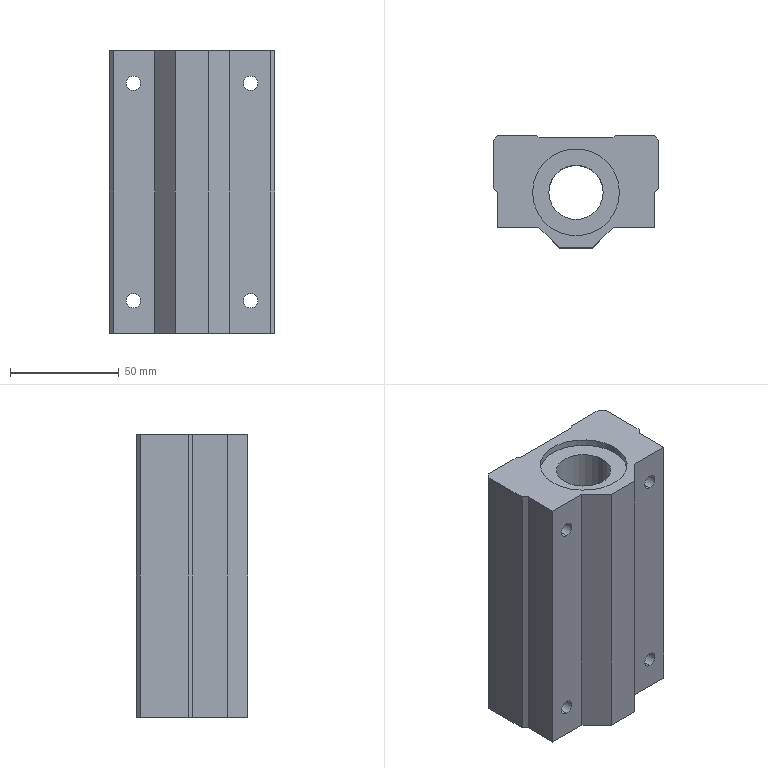Part | SolidWorks | features BaseBody 1 | 1 solid | 44 faces | box 76 x 51.5 x 130 mm | volume 357296 mm3 | plane 22 | cylinder 14 | cone 8 | commonest cylinder face diameters 6.647 x8 40 x4 25 x2
STEP:
#1=CARTESIAN_POINT('',(-12.5,0.,-127.));
#2=VERTEX_POINT('',#1);
#3=CARTESIAN_POINT('',(12.5,0.,-127.));
#4=VERTEX_POINT('',#3);
#5=CARTESIAN_POINT('',(0.,0.,-127.));
#6=DIRECTION('',(0.,0.,1.));
#7=DIRECTION('',(1.,0.,0.));
#8=AXIS2_PLACEMENT_3D('',#5,#6,#7);
#9=CIRCLE('',#8,12.5);
#10=EDGE_CURVE('',#2,#4,#9,.T.);
#11=ORIENTED_EDGE('',*,*,#10,.F.);
#12=CARTESIAN_POINT('',(-12.5,0.,-3.));
#13=VERTEX_POINT('',#12);
#14=CARTESIAN_POINT('',(-12.5,0.,-130.));
#15=DIRECTION('',(0.,0.,1.));
#16=VECTOR('',#15,1000.);
#17=LINE('',#14,#16);
#18=EDGE_CURVE('',#2,#13,#17,.T.);
#19=ORIENTED_EDGE('',*,*,#18,.T.);
#20=CARTESIAN_POINT('',(12.5,0.,-3.));
#21=VERTEX_POINT('',#20);
#22=CARTESIAN_POINT('',(0.,0.,-3.));
#23=DIRECTION('',(0.,0.,-1.));
#24=DIRECTION('',(1.,0.,0.));
#25=AXIS2_PLACEMENT_3D('',#22,#23,#24);
#26=CIRCLE('',#25,12.5);
#27=EDGE_CURVE('',#21,#13,#26,.T.);
#28=ORIENTED_EDGE('',*,*,#27,.F.);
#29=CARTESIAN_POINT('',(12.5,0.,-130.));
#30=DIRECTION('',(0.,0.,1.));
#31=VECTOR('',#30,1000.);
#32=LINE('',#29,#31);
#33=EDGE_CURVE('',#4,#21,#32,.T.);
#34=ORIENTED_EDGE('',*,*,#33,.F.);
#35=EDGE_LOOP('',(#11,#19,#28,#34));
#36=FACE_OUTER_BOUND('',#35,.T.);
#37=CARTESIAN_POINT('',(0.,0.,-130.));
#38=DIRECTION('',(0.,0.,1.));
#39=DIRECTION('',(1.,0.,0.));
#40=AXIS2_PLACEMENT_3D('',#37,#38,#39);
#41=CYLINDRICAL_SURFACE('',#40,12.5);
#42=ADVANCED_FACE('',(#36),#41,.F.);
#43=CARTESIAN_POINT('',(-20.,0.,-3.));
#44=VERTEX_POINT('',#43);
#45=CARTESIAN_POINT('',(20.,0.,-3.));
#46=VERTEX_POINT('',#45);
#47=CARTESIAN_POINT('',(0.,0.,-3.));
#48=DIRECTION('',(0.,0.,1.));
#49=DIRECTION('',(1.,0.,0.));
#50=AXIS2_PLACEMENT_3D('',#47,#48,#49);
#51=CIRCLE('',#50,20.);
#52=EDGE_CURVE('',#44,#46,#51,.T.);
#53=ORIENTED_EDGE('',*,*,#52,.F.);
#54=CARTESIAN_POINT('',(-20.,0.,0.));
#55=VERTEX_POINT('',#54);
#56=CARTESIAN_POINT('',(-20.,0.,-130.));
#57=DIRECTION('',(0.,0.,1.));
#58=VECTOR('',#57,1000.);
#59=LINE('',#56,#58);
#60=EDGE_CURVE('',#44,#55,#59,.T.);
#61=ORIENTED_EDGE('',*,*,#60,.T.);
#62=CARTESIAN_POINT('',(20.,0.,0.));
#63=VERTEX_POINT('',#62);
#64=CARTESIAN_POINT('',(0.,0.,0.));
#65=DIRECTION('',(0.,0.,-1.));
#66=DIRECTION('',(1.,0.,0.));
#67=AXIS2_PLACEMENT_3D('',#64,#65,#66);
#68=CIRCLE('',#67,20.);
#69=EDGE_CURVE('',#63,#55,#68,.T.);
#70=ORIENTED_EDGE('',*,*,#69,.F.);
#71=CARTESIAN_POINT('',(20.,0.,-130.));
#72=DIRECTION('',(0.,0.,1.));
#73=VECTOR('',#72,1000.);
#74=LINE('',#71,#73);
#75=EDGE_CURVE('',#46,#63,#74,.T.);
#76=ORIENTED_EDGE('',*,*,#75,.F.);
#77=EDGE_LOOP('',(#53,#61,#70,#76));
#78=FACE_OUTER_BOUND('',#77,.T.);
#79=CARTESIAN_POINT('',(0.,0.,-130.));
#80=DIRECTION('',(0.,0.,1.));
#81=DIRECTION('',(1.,0.,0.));
#82=AXIS2_PLACEMENT_3D('',#79,#80,#81);
#83=CYLINDRICAL_SURFACE('',#82,20.);
#84=ADVANCED_FACE('',(#78),#83,.F.);
#85=CARTESIAN_POINT('',(-20.,0.,-130.));
#86=VERTEX_POINT('',#85);
#87=CARTESIAN_POINT('',(20.,0.,-130.));
#88=VERTEX_POINT('',#87);
#89=CARTESIAN_POINT('',(0.,0.,-130.));
#90=DIRECTION('',(0.,0.,1.));
#91=DIRECTION('',(1.,0.,0.));
#92=AXIS2_PLACEMENT_3D('',#89,#90,#91);
#93=CIRCLE('',#92,20.);
#94=EDGE_CURVE('',#86,#88,#93,.T.);
#95=ORIENTED_EDGE('',*,*,#94,.F.);
#96=CARTESIAN_POINT('',(-20.,0.,-127.));
#97=VERTEX_POINT('',#96);
#98=CARTESIAN_POINT('',(-20.,0.,-130.));
#99=DIRECTION('',(0.,0.,1.));
#100=VECTOR('',#99,1000.);
#101=LINE('',#98,#100);
#102=EDGE_CURVE('',#86,#97,#101,.T.);
#103=ORIENTED_EDGE('',*,*,#102,.T.);
#104=CARTESIAN_POINT('',(20.,0.,-127.));
#105=VERTEX_POINT('',#104);
#106=CARTESIAN_POINT('',(0.,0.,-127.));
#107=DIRECTION('',(0.,0.,-1.));
#108=DIRECTION('',(1.,0.,0.));
#109=AXIS2_PLACEMENT_3D('',#106,#107,#108);
#110=CIRCLE('',#109,20.);
#111=EDGE_CURVE('',#105,#97,#110,.T.);
#112=ORIENTED_EDGE('',*,*,#111,.F.);
#113=CARTESIAN_POINT('',(20.,0.,-130.));
#114=DIRECTION('',(0.,0.,1.));
#115=VECTOR('',#114,1000.);
#116=LINE('',#113,#115);
#117=EDGE_CURVE('',#88,#105,#116,.T.);
#118=ORIENTED_EDGE('',*,*,#117,.F.);
#119=EDGE_LOOP('',(#95,#103,#112,#118));
#120=FACE_OUTER_BOUND('',#119,.T.);
#121=CARTESIAN_POINT('',(0.,0.,-130.));
#122=DIRECTION('',(0.,0.,1.));
#123=DIRECTION('',(1.,0.,0.));
#124=AXIS2_PLACEMENT_3D('',#121,#122,#123);
#125=CYLINDRICAL_SURFACE('',#124,20.);
#126=ADVANCED_FACE('',(#120),#125,.F.);
#127=CARTESIAN_POINT('',(-27.,25.323,-118.323));
#128=VERTEX_POINT('',#127);
#129=CARTESIAN_POINT('',(-27.,25.323,-111.677));
#130=VERTEX_POINT('',#129);
#131=CARTESIAN_POINT('',(-27.,25.323,-115.));
#132=DIRECTION('',(0.,1.,0.));
#133=DIRECTION('',(0.,0.,1.));
#134=AXIS2_PLACEMENT_3D('',#131,#132,#133);
#135=CIRCLE('',#134,3.323);
#136=EDGE_CURVE('',#128,#130,#135,.T.);
#137=ORIENTED_EDGE('',*,*,#136,.F.);
#138=CARTESIAN_POINT('',(-27.,26.,-119.));
#139=VERTEX_POINT('',#138);
#140=CARTESIAN_POINT('',(-27.,26.,-119.));
#141=DIRECTION('',(0.,0.7071,-0.7071));
#142=VECTOR('',#141,1000.);
#143=LINE('',#140,#142);
#144=EDGE_CURVE('',#128,#139,#143,.T.);
#145=ORIENTED_EDGE('',*,*,#144,.T.);
#146=CARTESIAN_POINT('',(-27.,26.,-111.));
#147=VERTEX_POINT('',#146);
#148=CARTESIAN_POINT('',(-27.,26.,-115.));
#149=DIRECTION('',(0.,-1.,0.));
#150=DIRECTION('',(0.,0.,1.));
#151=AXIS2_PLACEMENT_3D('',#148,#149,#150);
#152=CIRCLE('',#151,4.);
#153=EDGE_CURVE('',#147,#139,#152,.T.);
#154=ORIENTED_EDGE('',*,*,#153,.F.);
#155=CARTESIAN_POINT('',(-27.,26.,-111.));
#156=DIRECTION('',(0.,0.7071,0.7071));
#157=VECTOR('',#156,1000.);
#158=LINE('',#155,#157);
#159=EDGE_CURVE('',#130,#147,#158,.T.);
#160=ORIENTED_EDGE('',*,*,#159,.F.);
#161=EDGE_LOOP('',(#137,#145,#154,#160));
#162=FACE_OUTER_BOUND('',#161,.T.);
#163=CARTESIAN_POINT('',(-27.,26.,-115.));
#164=DIRECTION('',(0.,1.,0.));
#165=DIRECTION('',(0.,0.,1.));
#166=AXIS2_PLACEMENT_3D('',#163,#164,#165);
#167=CONICAL_SURFACE('',#166,4.,0.7854);
#168=ADVANCED_FACE('',(#162),#167,.F.);
#169=CARTESIAN_POINT('',(-27.,25.324,-18.324));
#170=VERTEX_POINT('',#169);
#171=CARTESIAN_POINT('',(-27.,25.324,-11.676));
#172=VERTEX_POINT('',#171);
#173=CARTESIAN_POINT('',(-27.,25.324,-15.));
#174=DIRECTION('',(0.,1.,0.));
#175=DIRECTION('',(0.,0.,1.));
#176=AXIS2_PLACEMENT_3D('',#173,#174,#175);
#177=CIRCLE('',#176,3.324);
#178=EDGE_CURVE('',#170,#172,#177,.T.);
#179=ORIENTED_EDGE('',*,*,#178,.F.);
#180=CARTESIAN_POINT('',(-27.,26.,-19.));
#181=VERTEX_POINT('',#180);
#182=CARTESIAN_POINT('',(-27.,26.,-19.));
#183=DIRECTION('',(0.,0.7071,-0.7071));
#184=VECTOR('',#183,1000.);
#185=LINE('',#182,#184);
#186=EDGE_CURVE('',#170,#181,#185,.T.);
#187=ORIENTED_EDGE('',*,*,#186,.T.);
#188=CARTESIAN_POINT('',(-27.,26.,-11.));
#189=VERTEX_POINT('',#188);
#190=CARTESIAN_POINT('',(-27.,26.,-15.));
#191=DIRECTION('',(0.,-1.,0.));
#192=DIRECTION('',(0.,0.,1.));
#193=AXIS2_PLACEMENT_3D('',#190,#191,#192);
#194=CIRCLE('',#193,4.);
#195=EDGE_CURVE('',#189,#181,#194,.T.);
#196=ORIENTED_EDGE('',*,*,#195,.F.);
#197=CARTESIAN_POINT('',(-27.,26.,-11.));
#198=DIRECTION('',(0.,0.7071,0.7071));
#199=VECTOR('',#198,1000.);
#200=LINE('',#197,#199);
#201=EDGE_CURVE('',#172,#189,#200,.T.);
#202=ORIENTED_EDGE('',*,*,#201,.F.);
#203=EDGE_LOOP('',(#179,#187,#196,#202));
#204=FACE_OUTER_BOUND('',#203,.T.);
#205=CARTESIAN_POINT('',(-27.,26.,-15.));
#206=DIRECTION('',(0.,1.,0.));
#207=DIRECTION('',(0.,0.,1.));
#208=AXIS2_PLACEMENT_3D('',#205,#206,#207);
#209=CONICAL_SURFACE('',#208,4.,0.7854);
#210=ADVANCED_FACE('',(#204),#209,.F.);
#211=CARTESIAN_POINT('',(27.,25.324,-118.324));
#212=VERTEX_POINT('',#211);
#213=CARTESIAN_POINT('',(27.,25.324,-111.676));
#214=VERTEX_POINT('',#213);
#215=CARTESIAN_POINT('',(27.,25.324,-115.));
#216=DIRECTION('',(0.,1.,0.));
#217=DIRECTION('',(0.,0.,1.));
#218=AXIS2_PLACEMENT_3D('',#215,#216,#217);
#219=CIRCLE('',#218,3.324);
#220=EDGE_CURVE('',#212,#214,#219,.T.);
#221=ORIENTED_EDGE('',*,*,#220,.F.);
#222=CARTESIAN_POINT('',(27.,26.,-119.));
#223=VERTEX_POINT('',#222);
#224=CARTESIAN_POINT('',(27.,26.,-119.));
#225=DIRECTION('',(0.,0.7071,-0.7071));
#226=VECTOR('',#225,1000.);
#227=LINE('',#224,#226);
#228=EDGE_CURVE('',#212,#223,#227,.T.);
#229=ORIENTED_EDGE('',*,*,#228,.T.);
#230=CARTESIAN_POINT('',(27.,26.,-111.));
#231=VERTEX_POINT('',#230);
#232=CARTESIAN_POINT('',(27.,26.,-115.));
#233=DIRECTION('',(0.,-1.,0.));
#234=DIRECTION('',(0.,0.,1.));
#235=AXIS2_PLACEMENT_3D('',#232,#233,#234);
#236=CIRCLE('',#235,4.);
#237=EDGE_CURVE('',#231,#223,#236,.T.);
#238=ORIENTED_EDGE('',*,*,#237,.F.);
#239=CARTESIAN_POINT('',(27.,26.,-111.));
#240=DIRECTION('',(0.,0.7071,0.7071));
#241=VECTOR('',#240,1000.);
#242=LINE('',#239,#241);
#243=EDGE_CURVE('',#214,#231,#242,.T.);
#244=ORIENTED_EDGE('',*,*,#243,.F.);
#245=EDGE_LOOP('',(#221,#229,#238,#244));
#246=FACE_OUTER_BOUND('',#245,.T.);
#247=CARTESIAN_POINT('',(27.,26.,-115.));
#248=DIRECTION('',(0.,1.,0.));
#249=DIRECTION('',(0.,0.,1.));
#250=AXIS2_PLACEMENT_3D('',#247,#248,#249);
#251=CONICAL_SURFACE('',#250,4.,0.7854);
#252=ADVANCED_FACE('',(#246),#251,.F.);
#253=CARTESIAN_POINT('',(27.,25.323,-18.323));
#254=VERTEX_POINT('',#253);
#255=CARTESIAN_POINT('',(27.,25.323,-11.677));
#256=VERTEX_POINT('',#255);
#257=CARTESIAN_POINT('',(27.,25.323,-15.));
#258=DIRECTION('',(0.,1.,0.));
#259=DIRECTION('',(0.,0.,1.));
#260=AXIS2_PLACEMENT_3D('',#257,#258,#259);
#261=CIRCLE('',#260,3.323);
#262=EDGE_CURVE('',#254,#256,#261,.T.);
#263=ORIENTED_EDGE('',*,*,#262,.F.);
#264=CARTESIAN_POINT('',(27.,26.,-19.));
#265=VERTEX_POINT('',#264);
#266=CARTESIAN_POINT('',(27.,26.,-19.));
#267=DIRECTION('',(0.,0.7071,-0.7071));
#268=VECTOR('',#267,1000.);
#269=LINE('',#266,#268);
#270=EDGE_CURVE('',#254,#265,#269,.T.);
#271=ORIENTED_EDGE('',*,*,#270,.T.);
#272=CARTESIAN_POINT('',(27.,26.,-11.));
#273=VERTEX_POINT('',#272);
#274=CARTESIAN_POINT('',(27.,26.,-15.));
#275=DIRECTION('',(0.,-1.,0.));
#276=DIRECTION('',(0.,0.,1.));
#277=AXIS2_PLACEMENT_3D('',#274,#275,#276);
#278=CIRCLE('',#277,4.);
#279=EDGE_CURVE('',#273,#265,#278,.T.);
#280=ORIENTED_EDGE('',*,*,#279,.F.);
#281=CARTESIAN_POINT('',(27.,26.,-11.));
#282=DIRECTION('',(0.,0.7071,0.7071));
#283=VECTOR('',#282,1000.);
#284=LINE('',#281,#283);
#285=EDGE_CURVE('',#256,#273,#284,.T.);
#286=ORIENTED_EDGE('',*,*,#285,.F.);
#287=EDGE_LOOP('',(#263,#271,#280,#286));
#288=FACE_OUTER_BOUND('',#287,.T.);
#289=CARTESIAN_POINT('',(27.,26.,-15.));
#290=DIRECTION('',(0.,1.,0.));
#291=DIRECTION('',(0.,0.,1.));
#292=AXIS2_PLACEMENT_3D('',#289,#290,#291);
#293=CONICAL_SURFACE('',#292,4.,0.7854);
#294=ADVANCED_FACE('',(#288),#293,.F.);
#295=CARTESIAN_POINT('',(27.,-16.,-118.323));
#296=VERTEX_POINT('',#295);
#297=CARTESIAN_POINT('',(27.,-16.,-111.677));
#298=VERTEX_POINT('',#297);
#299=CARTESIAN_POINT('',(27.,-16.,-115.));
#300=DIRECTION('',(0.,1.,0.));
#301=DIRECTION('',(0.,0.,1.));
#302=AXIS2_PLACEMENT_3D('',#299,#300,#301);
#303=CIRCLE('',#302,3.323);
#304=EDGE_CURVE('',#296,#298,#303,.T.);
#305=ORIENTED_EDGE('',*,*,#304,.F.);
#306=CARTESIAN_POINT('',(27.,-16.,-118.323));
#307=DIRECTION('',(0.,1.,0.));
#308=VECTOR('',#307,1000.);
#309=LINE('',#306,#308);
#310=EDGE_CURVE('',#296,#212,#309,.T.);
#311=ORIENTED_EDGE('',*,*,#310,.T.);
#312=ORIENTED_EDGE('',*,*,#220,.T.);
#313=CARTESIAN_POINT('',(27.,-16.,-111.677));
#314=DIRECTION('',(0.,1.,0.));
#315=VECTOR('',#314,1000.);
#316=LINE('',#313,#315);
#317=EDGE_CURVE('',#298,#214,#316,.T.);
#318=ORIENTED_EDGE('',*,*,#317,.F.);
#319=EDGE_LOOP('',(#305,#311,#312,#318));
#320=FACE_OUTER_BOUND('',#319,.T.);
#321=CARTESIAN_POINT('',(27.,-16.,-115.));
#322=DIRECTION('',(0.,1.,0.));
#323=DIRECTION('',(0.,0.,1.));
#324=AXIS2_PLACEMENT_3D('',#321,#322,#323);
#325=CYLINDRICAL_SURFACE('',#324,3.323);
#326=ADVANCED_FACE('',(#320),#325,.F.);
#327=CARTESIAN_POINT('',(27.,-16.,-18.323));
#328=VERTEX_POINT('',#327);
#329=CARTESIAN_POINT('',(27.,-16.,-11.676));
#330=VERTEX_POINT('',#329);
#331=CARTESIAN_POINT('',(27.,-16.,-15.));
#332=DIRECTION('',(0.,1.,0.));
#333=DIRECTION('',(0.,0.,1.));
#334=AXIS2_PLACEMENT_3D('',#331,#332,#333);
#335=CIRCLE('',#334,3.324);
#336=EDGE_CURVE('',#328,#330,#335,.T.);
#337=ORIENTED_EDGE('',*,*,#336,.F.);
#338=CARTESIAN_POINT('',(27.,-16.,-18.323));
#339=DIRECTION('',(0.,1.,0.));
#340=VECTOR('',#339,1000.);
#341=LINE('',#338,#340);
#342=EDGE_CURVE('',#328,#254,#341,.T.);
#343=ORIENTED_EDGE('',*,*,#342,.T.);
#344=ORIENTED_EDGE('',*,*,#262,.T.);
#345=CARTESIAN_POINT('',(27.,-16.,-11.676));
#346=DIRECTION('',(0.,1.,0.));
#347=VECTOR('',#346,1000.);
#348=LINE('',#345,#347);
#349=EDGE_CURVE('',#330,#256,#348,.T.);
#350=ORIENTED_EDGE('',*,*,#349,.F.);
#351=EDGE_LOOP('',(#337,#343,#344,#350));
#352=FACE_OUTER_BOUND('',#351,.T.);
#353=CARTESIAN_POINT('',(27.,-16.,-15.));
#354=DIRECTION('',(0.,1.,0.));
#355=DIRECTION('',(0.,0.,1.));
#356=AXIS2_PLACEMENT_3D('',#353,#354,#355);
#357=CYLINDRICAL_SURFACE('',#356,3.324);
#358=ADVANCED_FACE('',(#352),#357,.F.);
#359=ORIENTED_EDGE('',*,*,#136,.T.);
#360=CARTESIAN_POINT('',(-27.,-16.,-111.677));
#361=VERTEX_POINT('',#360);
#362=CARTESIAN_POINT('',(-27.,26.,-111.677));
#363=DIRECTION('',(0.,-1.,0.));
#364=VECTOR('',#363,1000.);
#365=LINE('',#362,#364);
#366=EDGE_CURVE('',#130,#361,#365,.T.);
#367=ORIENTED_EDGE('',*,*,#366,.T.);
#368=CARTESIAN_POINT('',(-27.,-16.,-118.323));
#369=VERTEX_POINT('',#368);
#370=CARTESIAN_POINT('',(-27.,-16.,-115.));
#371=DIRECTION('',(0.,1.,0.));
#372=DIRECTION('',(0.,0.,-1.));
#373=AXIS2_PLACEMENT_3D('',#370,#371,#372);
#374=CIRCLE('',#373,3.323);
#375=EDGE_CURVE('',#369,#361,#374,.T.);
#376=ORIENTED_EDGE('',*,*,#375,.F.);
#377=CARTESIAN_POINT('',(-27.,26.,-118.323));
#378=DIRECTION('',(0.,-1.,0.));
#379=VECTOR('',#378,1000.);
#380=LINE('',#377,#379);
#381=EDGE_CURVE('',#128,#369,#380,.T.);
#382=ORIENTED_EDGE('',*,*,#381,.F.);
#383=EDGE_LOOP('',(#359,#367,#376,#382));
#384=FACE_OUTER_BOUND('',#383,.T.);
#385=CARTESIAN_POINT('',(-27.,26.,-115.));
#386=DIRECTION('',(0.,-1.,0.));
#387=DIRECTION('',(0.,0.,-1.));
#388=AXIS2_PLACEMENT_3D('',#385,#386,#387);
#389=CYLINDRICAL_SURFACE('',#388,3.323);
#390=ADVANCED_FACE('',(#384),#389,.F.);
#391=ORIENTED_EDGE('',*,*,#178,.T.);
#392=CARTESIAN_POINT('',(-27.,-16.,-11.676));
#393=VERTEX_POINT('',#392);
#394=CARTESIAN_POINT('',(-27.,26.,-11.676));
#395=DIRECTION('',(0.,-1.,0.));
#396=VECTOR('',#395,1000.);
#397=LINE('',#394,#396);
#398=EDGE_CURVE('',#172,#393,#397,.T.);
#399=ORIENTED_EDGE('',*,*,#398,.T.);
#400=CARTESIAN_POINT('',(-27.,-16.,-18.323));
#401=VERTEX_POINT('',#400);
#402=CARTESIAN_POINT('',(-27.,-16.,-15.));
#403=DIRECTION('',(0.,1.,0.));
#404=DIRECTION('',(0.,0.,-1.));
#405=AXIS2_PLACEMENT_3D('',#402,#403,#404);
#406=CIRCLE('',#405,3.324);
#407=EDGE_CURVE('',#401,#393,#406,.T.);
#408=ORIENTED_EDGE('',*,*,#407,.F.);
#409=CARTESIAN_POINT('',(-27.,26.,-18.323));
#410=DIRECTION('',(0.,-1.,0.));
#411=VECTOR('',#410,1000.);
#412=LINE('',#409,#411);
#413=EDGE_CURVE('',#170,#401,#412,.T.);
#414=ORIENTED_EDGE('',*,*,#413,.F.);
#415=EDGE_LOOP('',(#391,#399,#408,#414));
#416=FACE_OUTER_BOUND('',#415,.T.);
#417=CARTESIAN_POINT('',(-27.,26.,-15.));
#418=DIRECTION('',(0.,-1.,0.));
#419=DIRECTION('',(0.,0.,-1.));
#420=AXIS2_PLACEMENT_3D('',#417,#418,#419);
#421=CYLINDRICAL_SURFACE('',#420,3.324);
#422=ADVANCED_FACE('',(#416),#421,.F.);
#423=ORIENTED_EDGE('',*,*,#18,.F.);
#424=CARTESIAN_POINT('',(0.,0.,-127.));
#425=DIRECTION('',(0.,0.,1.));
#426=DIRECTION('',(1.,0.,0.));
#427=AXIS2_PLACEMENT_3D('',#424,#425,#426);
#428=CIRCLE('',#427,12.5);
#429=EDGE_CURVE('',#4,#2,#428,.T.);
#430=ORIENTED_EDGE('',*,*,#429,.F.);
#431=ORIENTED_EDGE('',*,*,#33,.T.);
#432=CARTESIAN_POINT('',(0.,0.,-3.));
#433=DIRECTION('',(0.,0.,-1.));
#434=DIRECTION('',(1.,0.,0.));
#435=AXIS2_PLACEMENT_3D('',#432,#433,#434);
#436=CIRCLE('',#435,12.5);
#437=EDGE_CURVE('',#13,#21,#436,.T.);
#438=ORIENTED_EDGE('',*,*,#437,.F.);
#439=EDGE_LOOP('',(#423,#430,#431,#438));
#440=FACE_OUTER_BOUND('',#439,.T.);
#441=CARTESIAN_POINT('',(0.,0.,-130.));
#442=DIRECTION('',(0.,0.,1.));
#443=DIRECTION('',(1.,0.,0.));
#444=AXIS2_PLACEMENT_3D('',#441,#442,#443);
#445=CYLINDRICAL_SURFACE('',#444,12.5);
#446=ADVANCED_FACE('',(#440),#445,.F.);
#447=CARTESIAN_POINT('',(0.,0.,-3.));
#448=DIRECTION('',(0.,0.,1.));
#449=DIRECTION('',(1.,0.,0.));
#450=AXIS2_PLACEMENT_3D('',#447,#448,#449);
#451=CIRCLE('',#450,20.);
#452=EDGE_CURVE('',#46,#44,#451,.T.);
#453=ORIENTED_EDGE('',*,*,#452,.T.);
#454=ORIENTED_EDGE('',*,*,#52,.T.);
#455=EDGE_LOOP('',(#453,#454));
#456=FACE_OUTER_BOUND('',#455,.T.);
#457=ORIENTED_EDGE('',*,*,#27,.T.);
#458=ORIENTED_EDGE('',*,*,#437,.T.);
#459=EDGE_LOOP('',(#457,#458));
#460=FACE_BOUND('',#459,.T.);
#461=CARTESIAN_POINT('',(0.,20.,-3.));
#462=DIRECTION('',(0.,0.,1.));
#463=DIRECTION('',(1.,0.,0.));
#464=AXIS2_PLACEMENT_3D('',#461,#462,#463);
#465=PLANE('',#464);
#466=ADVANCED_FACE('',(#456,#460),#465,.T.);
#467=ORIENTED_EDGE('',*,*,#429,.T.);
#468=ORIENTED_EDGE('',*,*,#10,.T.);
#469=EDGE_LOOP('',(#467,#468));
#470=FACE_BOUND('',#469,.T.);
#471=ORIENTED_EDGE('',*,*,#111,.T.);
#472=CARTESIAN_POINT('',(0.,0.,-127.));
#473=DIRECTION('',(0.,0.,-1.));
#474=DIRECTION('',(1.,0.,0.));
#475=AXIS2_PLACEMENT_3D('',#472,#473,#474);
#476=CIRCLE('',#475,20.);
#477=EDGE_CURVE('',#97,#105,#476,.T.);
#478=ORIENTED_EDGE('',*,*,#477,.T.);
#479=EDGE_LOOP('',(#471,#478));
#480=FACE_OUTER_BOUND('',#479,.T.);
#481=CARTESIAN_POINT('',(0.,12.5,-127.));
#482=DIRECTION('',(0.,0.,-1.));
#483=DIRECTION('',(-1.,0.,0.));
#484=AXIS2_PLACEMENT_3D('',#481,#482,#483);
#485=PLANE('',#484);
#486=ADVANCED_FACE('',(#470,#480),#485,.T.);
#487=ORIENTED_EDGE('',*,*,#60,.F.);
#488=ORIENTED_EDGE('',*,*,#452,.F.);
#489=ORIENTED_EDGE('',*,*,#75,.T.);
#490=CARTESIAN_POINT('',(0.,0.,0.));
#491=DIRECTION('',(0.,0.,-1.));
#492=DIRECTION('',(1.,0.,0.));
#493=AXIS2_PLACEMENT_3D('',#490,#491,#492);
#494=CIRCLE('',#493,20.);
#495=EDGE_CURVE('',#55,#63,#494,.T.);
#496=ORIENTED_EDGE('',*,*,#495,.F.);
#497=EDGE_LOOP('',(#487,#488,#489,#496));
#498=FACE_OUTER_BOUND('',#497,.T.);
#499=CARTESIAN_POINT('',(0.,0.,-130.));
#500=DIRECTION('',(0.,0.,1.));
#501=DIRECTION('',(1.,0.,0.));
#502=AXIS2_PLACEMENT_3D('',#499,#500,#501);
#503=CYLINDRICAL_SURFACE('',#502,20.);
#504=ADVANCED_FACE('',(#498),#503,.F.);
#505=ORIENTED_EDGE('',*,*,#102,.F.);
#506=CARTESIAN_POINT('',(0.,0.,-130.));
#507=DIRECTION('',(0.,0.,1.));
#508=DIRECTION('',(1.,0.,0.));
#509=AXIS2_PLACEMENT_3D('',#506,#507,#508);
#510=CIRCLE('',#509,20.);
#511=EDGE_CURVE('',#88,#86,#510,.T.);
#512=ORIENTED_EDGE('',*,*,#511,.F.);
#513=ORIENTED_EDGE('',*,*,#117,.T.);
#514=ORIENTED_EDGE('',*,*,#477,.F.);
#515=EDGE_LOOP('',(#505,#512,#513,#514));
#516=FACE_OUTER_BOUND('',#515,.T.);
#517=CARTESIAN_POINT('',(0.,0.,-130.));
#518=DIRECTION('',(0.,0.,1.));
#519=DIRECTION('',(1.,0.,0.));
#520=AXIS2_PLACEMENT_3D('',#517,#518,#519);
#521=CYLINDRICAL_SURFACE('',#520,20.);
#522=ADVANCED_FACE('',(#516),#521,.F.);
#523=ORIENTED_EDGE('',*,*,#69,.T.);
#524=ORIENTED_EDGE('',*,*,#495,.T.);
#525=EDGE_LOOP('',(#523,#524));
#526=FACE_BOUND('',#525,.T.);
#527=CARTESIAN_POINT('',(-18.,26.,0.));
#528=VERTEX_POINT('',#527);
#529=CARTESIAN_POINT('',(-36.,26.,0.));
#530=VERTEX_POINT('',#529);
#531=CARTESIAN_POINT('',(0.,26.,0.));
#532=DIRECTION('',(-1.,0.,0.));
#533=VECTOR('',#532,1000.);
#534=LINE('',#531,#533);
#535=EDGE_CURVE('',#528,#530,#534,.T.);
#536=ORIENTED_EDGE('',*,*,#535,.T.);
#537=CARTESIAN_POINT('',(-38.,24.,0.));
#538=VERTEX_POINT('',#537);
#539=CARTESIAN_POINT('',(-36.,26.,0.));
#540=DIRECTION('',(-0.7071,-0.7071,0.));
#541=VECTOR('',#540,1000.);
#542=LINE('',#539,#541);
#543=EDGE_CURVE('',#530,#538,#542,.T.);
#544=ORIENTED_EDGE('',*,*,#543,.T.);
#545=CARTESIAN_POINT('',(-38.,2.,0.));
#546=VERTEX_POINT('',#545);
#547=CARTESIAN_POINT('',(-38.,0.,0.));
#548=DIRECTION('',(0.,-1.,0.));
#549=VECTOR('',#548,1000.);
#550=LINE('',#547,#549);
#551=EDGE_CURVE('',#538,#546,#550,.T.);
#552=ORIENTED_EDGE('',*,*,#551,.T.);
#553=CARTESIAN_POINT('',(-36.,0.,0.));
#554=VERTEX_POINT('',#553);
#555=CARTESIAN_POINT('',(-38.,2.,0.));
#556=DIRECTION('',(0.7071,-0.7071,0.));
#557=VECTOR('',#556,1000.);
#558=LINE('',#555,#557);
#559=EDGE_CURVE('',#546,#554,#558,.T.);
#560=ORIENTED_EDGE('',*,*,#559,.T.);
#561=CARTESIAN_POINT('',(-36.,-16.,0.));
#562=VERTEX_POINT('',#561);
#563=CARTESIAN_POINT('',(-36.,0.,0.));
#564=DIRECTION('',(0.,-1.,0.));
#565=VECTOR('',#564,1000.);
#566=LINE('',#563,#565);
#567=EDGE_CURVE('',#554,#562,#566,.T.);
#568=ORIENTED_EDGE('',*,*,#567,.T.);
#569=CARTESIAN_POINT('',(-17.1,-16.,0.));
#570=VERTEX_POINT('',#569);
#571=CARTESIAN_POINT('',(0.,-16.,0.));
#572=DIRECTION('',(1.,0.,0.));
#573=VECTOR('',#572,1000.);
#574=LINE('',#571,#573);
#575=EDGE_CURVE('',#562,#570,#574,.T.);
#576=ORIENTED_EDGE('',*,*,#575,.T.);
#577=CARTESIAN_POINT('',(-7.6,-25.5,0.));
#578=VERTEX_POINT('',#577);
#579=CARTESIAN_POINT('',(-17.1,-16.,0.));
#580=DIRECTION('',(0.7071,-0.7071,0.));
#581=VECTOR('',#580,1000.);
#582=LINE('',#579,#581);
#583=EDGE_CURVE('',#570,#578,#582,.T.);
#584=ORIENTED_EDGE('',*,*,#583,.T.);
#585=CARTESIAN_POINT('',(7.6,-25.5,0.));
#586=VERTEX_POINT('',#585);
#587=CARTESIAN_POINT('',(0.,-25.5,0.));
#588=DIRECTION('',(1.,0.,0.));
#589=VECTOR('',#588,1000.);
#590=LINE('',#587,#589);
#591=EDGE_CURVE('',#578,#586,#590,.T.);
#592=ORIENTED_EDGE('',*,*,#591,.T.);
#593=CARTESIAN_POINT('',(17.1,-16.,0.));
#594=VERTEX_POINT('',#593);
#595=CARTESIAN_POINT('',(7.6,-25.5,0.));
#596=DIRECTION('',(0.7071,0.7071,0.));
#597=VECTOR('',#596,1000.);
#598=LINE('',#595,#597);
#599=EDGE_CURVE('',#586,#594,#598,.T.);
#600=ORIENTED_EDGE('',*,*,#599,.T.);
#601=CARTESIAN_POINT('',(36.,-16.,0.));
#602=VERTEX_POINT('',#601);
#603=CARTESIAN_POINT('',(0.,-16.,0.));
#604=DIRECTION('',(1.,0.,0.));
#605=VECTOR('',#604,1000.);
#606=LINE('',#603,#605);
#607=EDGE_CURVE('',#594,#602,#606,.T.);
#608=ORIENTED_EDGE('',*,*,#607,.T.);
#609=CARTESIAN_POINT('',(36.,0.,0.));
#610=VERTEX_POINT('',#609);
#611=CARTESIAN_POINT('',(36.,0.,0.));
#612=DIRECTION('',(0.,1.,0.));
#613=VECTOR('',#612,1000.);
#614=LINE('',#611,#613);
#615=EDGE_CURVE('',#602,#610,#614,.T.);
#616=ORIENTED_EDGE('',*,*,#615,.T.);
#617=CARTESIAN_POINT('',(38.,2.,0.));
#618=VERTEX_POINT('',#617);
#619=CARTESIAN_POINT('',(36.,0.,0.));
#620=DIRECTION('',(0.7071,0.7071,0.));
#621=VECTOR('',#620,1000.);
#622=LINE('',#619,#621);
#623=EDGE_CURVE('',#610,#618,#622,.T.);
#624=ORIENTED_EDGE('',*,*,#623,.T.);
#625=CARTESIAN_POINT('',(38.,24.,0.));
#626=VERTEX_POINT('',#625);
#627=CARTESIAN_POINT('',(38.,0.,0.));
#628=DIRECTION('',(0.,1.,0.));
#629=VECTOR('',#628,1000.);
#630=LINE('',#627,#629);
#631=EDGE_CURVE('',#618,#626,#630,.T.);
#632=ORIENTED_EDGE('',*,*,#631,.T.);
#633=CARTESIAN_POINT('',(36.,26.,0.));
#634=VERTEX_POINT('',#633);
#635=CARTESIAN_POINT('',(38.,24.,0.));
#636=DIRECTION('',(-0.7071,0.7071,0.));
#637=VECTOR('',#636,1000.);
#638=LINE('',#635,#637);
#639=EDGE_CURVE('',#626,#634,#638,.T.);
#640=ORIENTED_EDGE('',*,*,#639,.T.);
#641=CARTESIAN_POINT('',(18.,26.,0.));
#642=VERTEX_POINT('',#641);
#643=CARTESIAN_POINT('',(0.,26.,0.));
#644=DIRECTION('',(-1.,0.,0.));
#645=VECTOR('',#644,1000.);
#646=LINE('',#643,#645);
#647=EDGE_CURVE('',#634,#642,#646,.T.);
#648=ORIENTED_EDGE('',*,*,#647,.T.);
#649=CARTESIAN_POINT('',(17.,25.,0.));
#650=VERTEX_POINT('',#649);
#651=CARTESIAN_POINT('',(18.,26.,0.));
#652=DIRECTION('',(0.7071,0.7071,0.));
#653=VECTOR('',#652,1000.);
#654=LINE('',#651,#653);
#655=EDGE_CURVE('',#650,#642,#654,.T.);
#656=ORIENTED_EDGE('',*,*,#655,.F.);
#657=CARTESIAN_POINT('',(-17.,25.,0.));
#658=VERTEX_POINT('',#657);
#659=CARTESIAN_POINT('',(0.,25.,0.));
#660=DIRECTION('',(-1.,0.,0.));
#661=VECTOR('',#660,1000.);
#662=LINE('',#659,#661);
#663=EDGE_CURVE('',#650,#658,#662,.T.);
#664=ORIENTED_EDGE('',*,*,#663,.T.);
#665=CARTESIAN_POINT('',(-17.,25.,0.));
#666=DIRECTION('',(0.7071,-0.7071,0.));
#667=VECTOR('',#666,1000.);
#668=LINE('',#665,#667);
#669=EDGE_CURVE('',#528,#658,#668,.T.);
#670=ORIENTED_EDGE('',*,*,#669,.F.);
#671=EDGE_LOOP('',(#536,#544,#552,#560,#568,#576,#584,#592,#600,#608,#616,#624,#632,#640,#648,#656,#664,#670));
#672=FACE_OUTER_BOUND('',#671,.T.);
#673=CARTESIAN_POINT('',(0.,0.,0.));
#674=DIRECTION('',(0.,0.,1.));
#675=DIRECTION('',(1.,0.,0.));
#676=AXIS2_PLACEMENT_3D('',#673,#674,#675);
#677=PLANE('',#676);
#678=ADVANCED_FACE('',(#526,#672),#677,.T.);
#679=ORIENTED_EDGE('',*,*,#511,.T.);
#680=ORIENTED_EDGE('',*,*,#94,.T.);
#681=EDGE_LOOP('',(#679,#680));
#682=FACE_BOUND('',#681,.T.);
#683=CARTESIAN_POINT('',(-36.,26.,-130.));
#684=VERTEX_POINT('',#683);
#685=CARTESIAN_POINT('',(-38.,24.,-130.));
#686=VERTEX_POINT('',#685);
#687=CARTESIAN_POINT('',(-36.,26.,-130.));
#688=DIRECTION('',(-0.7071,-0.7071,0.));
#689=VECTOR('',#688,1000.);
#690=LINE('',#687,#689);
#691=EDGE_CURVE('',#684,#686,#690,.T.);
#692=ORIENTED_EDGE('',*,*,#691,.F.);
#693=CARTESIAN_POINT('',(-18.,26.,-130.));
#694=VERTEX_POINT('',#693);
#695=CARTESIAN_POINT('',(0.,26.,-130.));
#696=DIRECTION('',(-1.,0.,0.));
#697=VECTOR('',#696,1000.);
#698=LINE('',#695,#697);
#699=EDGE_CURVE('',#694,#684,#698,.T.);
#700=ORIENTED_EDGE('',*,*,#699,.F.);
#701=CARTESIAN_POINT('',(-17.,25.,-130.));
#702=VERTEX_POINT('',#701);
#703=CARTESIAN_POINT('',(-17.,25.,-130.));
#704=DIRECTION('',(-0.7071,0.7071,0.));
#705=VECTOR('',#704,1000.);
#706=LINE('',#703,#705);
#707=EDGE_CURVE('',#702,#694,#706,.T.);
#708=ORIENTED_EDGE('',*,*,#707,.F.);
#709=CARTESIAN_POINT('',(17.,25.,-130.));
#710=VERTEX_POINT('',#709);
#711=CARTESIAN_POINT('',(0.,25.,-130.));
#712=DIRECTION('',(-1.,0.,0.));
#713=VECTOR('',#712,1000.);
#714=LINE('',#711,#713);
#715=EDGE_CURVE('',#710,#702,#714,.T.);
#716=ORIENTED_EDGE('',*,*,#715,.F.);
#717=CARTESIAN_POINT('',(18.,26.,-130.));
#718=VERTEX_POINT('',#717);
#719=CARTESIAN_POINT('',(18.,26.,-130.));
#720=DIRECTION('',(-0.7071,-0.7071,0.));
#721=VECTOR('',#720,1000.);
#722=LINE('',#719,#721);
#723=EDGE_CURVE('',#718,#710,#722,.T.);
#724=ORIENTED_EDGE('',*,*,#723,.F.);
#725=CARTESIAN_POINT('',(36.,26.,-130.));
#726=VERTEX_POINT('',#725);
#727=CARTESIAN_POINT('',(0.,26.,-130.));
#728=DIRECTION('',(-1.,0.,0.));
#729=VECTOR('',#728,1000.);
#730=LINE('',#727,#729);
#731=EDGE_CURVE('',#726,#718,#730,.T.);
#732=ORIENTED_EDGE('',*,*,#731,.F.);
#733=CARTESIAN_POINT('',(38.,24.,-130.));
#734=VERTEX_POINT('',#733);
#735=CARTESIAN_POINT('',(38.,24.,-130.));
#736=DIRECTION('',(-0.7071,0.7071,0.));
#737=VECTOR('',#736,1000.);
#738=LINE('',#735,#737);
#739=EDGE_CURVE('',#734,#726,#738,.T.);
#740=ORIENTED_EDGE('',*,*,#739,.F.);
#741=CARTESIAN_POINT('',(38.,2.,-130.));
#742=VERTEX_POINT('',#741);
#743=CARTESIAN_POINT('',(38.,0.,-130.));
#744=DIRECTION('',(0.,1.,0.));
#745=VECTOR('',#744,1000.);
#746=LINE('',#743,#745);
#747=EDGE_CURVE('',#742,#734,#746,.T.);
#748=ORIENTED_EDGE('',*,*,#747,.F.);
#749=CARTESIAN_POINT('',(36.,0.,-130.));
#750=VERTEX_POINT('',#749);
#751=CARTESIAN_POINT('',(36.,0.,-130.));
#752=DIRECTION('',(0.7071,0.7071,0.));
#753=VECTOR('',#752,1000.);
#754=LINE('',#751,#753);
#755=EDGE_CURVE('',#750,#742,#754,.T.);
#756=ORIENTED_EDGE('',*,*,#755,.F.);
#757=CARTESIAN_POINT('',(36.,-16.,-130.));
#758=VERTEX_POINT('',#757);
#759=CARTESIAN_POINT('',(36.,0.,-130.));
#760=DIRECTION('',(0.,1.,0.));
#761=VECTOR('',#760,1000.);
#762=LINE('',#759,#761);
#763=EDGE_CURVE('',#758,#750,#762,.T.);
#764=ORIENTED_EDGE('',*,*,#763,.F.);
#765=CARTESIAN_POINT('',(17.1,-16.,-130.));
#766=VERTEX_POINT('',#765);
#767=CARTESIAN_POINT('',(0.,-16.,-130.));
#768=DIRECTION('',(1.,0.,0.));
#769=VECTOR('',#768,1000.);
#770=LINE('',#767,#769);
#771=EDGE_CURVE('',#766,#758,#770,.T.);
#772=ORIENTED_EDGE('',*,*,#771,.F.);
#773=CARTESIAN_POINT('',(7.6,-25.5,-130.));
#774=VERTEX_POINT('',#773);
#775=CARTESIAN_POINT('',(7.6,-25.5,-130.));
#776=DIRECTION('',(0.7071,0.7071,0.));
#777=VECTOR('',#776,1000.);
#778=LINE('',#775,#777);
#779=EDGE_CURVE('',#774,#766,#778,.T.);
#780=ORIENTED_EDGE('',*,*,#779,.F.);
#781=CARTESIAN_POINT('',(-7.6,-25.5,-130.));
#782=VERTEX_POINT('',#781);
#783=CARTESIAN_POINT('',(0.,-25.5,-130.));
#784=DIRECTION('',(1.,0.,0.));
#785=VECTOR('',#784,1000.);
#786=LINE('',#783,#785);
#787=EDGE_CURVE('',#782,#774,#786,.T.);
#788=ORIENTED_EDGE('',*,*,#787,.F.);
#789=CARTESIAN_POINT('',(-17.1,-16.,-130.));
#790=VERTEX_POINT('',#789);
#791=CARTESIAN_POINT('',(-17.1,-16.,-130.));
#792=DIRECTION('',(0.7071,-0.7071,0.));
#793=VECTOR('',#792,1000.);
#794=LINE('',#791,#793);
#795=EDGE_CURVE('',#790,#782,#794,.T.);
#796=ORIENTED_EDGE('',*,*,#795,.F.);
#797=CARTESIAN_POINT('',(-36.,-16.,-130.));
#798=VERTEX_POINT('',#797);
#799=CARTESIAN_POINT('',(0.,-16.,-130.));
#800=DIRECTION('',(1.,0.,0.));
#801=VECTOR('',#800,1000.);
#802=LINE('',#799,#801);
#803=EDGE_CURVE('',#798,#790,#802,.T.);
#804=ORIENTED_EDGE('',*,*,#803,.F.);
#805=CARTESIAN_POINT('',(-36.,0.,-130.));
#806=VERTEX_POINT('',#805);
#807=CARTESIAN_POINT('',(-36.,0.,-130.));
#808=DIRECTION('',(0.,-1.,0.));
#809=VECTOR('',#808,1000.);
#810=LINE('',#807,#809);
#811=EDGE_CURVE('',#806,#798,#810,.T.);
#812=ORIENTED_EDGE('',*,*,#811,.F.);
#813=CARTESIAN_POINT('',(-38.,2.,-130.));
#814=VERTEX_POINT('',#813);
#815=CARTESIAN_POINT('',(-38.,2.,-130.));
#816=DIRECTION('',(0.7071,-0.7071,0.));
#817=VECTOR('',#816,1000.);
#818=LINE('',#815,#817);
#819=EDGE_CURVE('',#814,#806,#818,.T.);
#820=ORIENTED_EDGE('',*,*,#819,.F.);
#821=CARTESIAN_POINT('',(-38.,0.,-130.));
#822=DIRECTION('',(0.,-1.,0.));
#823=VECTOR('',#822,1000.);
#824=LINE('',#821,#823);
#825=EDGE_CURVE('',#686,#814,#824,.T.);
#826=ORIENTED_EDGE('',*,*,#825,.F.);
#827=EDGE_LOOP('',(#692,#700,#708,#716,#724,#732,#740,#748,#756,#764,#772,#780,#788,#796,#804,#812,#820,#826));
#828=FACE_OUTER_BOUND('',#827,.T.);
#829=CARTESIAN_POINT('',(0.,0.,-130.));
#830=DIRECTION('',(0.,0.,1.));
#831=DIRECTION('',(1.,0.,0.));
#832=AXIS2_PLACEMENT_3D('',#829,#830,#831);
#833=PLANE('',#832);
#834=ADVANCED_FACE('',(#682,#828),#833,.F.);
#835=ORIENTED_EDGE('',*,*,#691,.T.);
#836=CARTESIAN_POINT('',(-38.,24.,-130.));
#837=DIRECTION('',(0.,0.,1.));
#838=VECTOR('',#837,1000.);
#839=LINE('',#836,#838);
#840=EDGE_CURVE('',#686,#538,#839,.T.);
#841=ORIENTED_EDGE('',*,*,#840,.T.);
#842=ORIENTED_EDGE('',*,*,#543,.F.);
#843=CARTESIAN_POINT('',(-36.,26.,-130.));
#844=DIRECTION('',(0.,0.,-1.));
#845=VECTOR('',#844,1000.);
#846=LINE('',#843,#845);
#847=EDGE_CURVE('',#530,#684,#846,.T.);
#848=ORIENTED_EDGE('',*,*,#847,.T.);
#849=EDGE_LOOP('',(#835,#841,#842,#848));
#850=FACE_OUTER_BOUND('',#849,.T.);
#851=CARTESIAN_POINT('',(-36.,26.,-130.));
#852=DIRECTION('',(-0.7071,0.7071,0.));
#853=DIRECTION('',(-0.7071,-0.7071,0.));
#854=AXIS2_PLACEMENT_3D('',#851,#852,#853);
#855=PLANE('',#854);
#856=ADVANCED_FACE('',(#850),#855,.T.);
#857=ORIENTED_EDGE('',*,*,#153,.T.);
#858=CARTESIAN_POINT('',(-27.,26.,-115.));
#859=DIRECTION('',(0.,-1.,0.));
#860=DIRECTION('',(0.,0.,1.));
#861=AXIS2_PLACEMENT_3D('',#858,#859,#860);
#862=CIRCLE('',#861,4.);
#863=EDGE_CURVE('',#139,#147,#862,.T.);
#864=ORIENTED_EDGE('',*,*,#863,.T.);
#865=EDGE_LOOP('',(#857,#864));
#866=FACE_BOUND('',#865,.T.);
#867=ORIENTED_EDGE('',*,*,#699,.T.);
#868=ORIENTED_EDGE('',*,*,#847,.F.);
#869=ORIENTED_EDGE('',*,*,#535,.F.);
#870=CARTESIAN_POINT('',(-18.,26.,-130.));
#871=DIRECTION('',(0.,0.,-1.));
#872=VECTOR('',#871,1000.);
#873=LINE('',#870,#872);
#874=EDGE_CURVE('',#528,#694,#873,.T.);
#875=ORIENTED_EDGE('',*,*,#874,.T.);
#876=EDGE_LOOP('',(#867,#868,#869,#875));
#877=FACE_OUTER_BOUND('',#876,.T.);
#878=ORIENTED_EDGE('',*,*,#195,.T.);
#879=CARTESIAN_POINT('',(-27.,26.,-15.));
#880=DIRECTION('',(0.,-1.,0.));
#881=DIRECTION('',(0.,0.,1.));
#882=AXIS2_PLACEMENT_3D('',#879,#880,#881);
#883=CIRCLE('',#882,4.);
#884=EDGE_CURVE('',#181,#189,#883,.T.);
#885=ORIENTED_EDGE('',*,*,#884,.T.);
#886=EDGE_LOOP('',(#878,#885));
#887=FACE_BOUND('',#886,.T.);
#888=CARTESIAN_POINT('',(-18.,26.,-130.));
#889=DIRECTION('',(0.,1.,0.));
#890=DIRECTION('',(0.,0.,1.));
#891=AXIS2_PLACEMENT_3D('',#888,#889,#890);
#892=PLANE('',#891);
#893=ADVANCED_FACE('',(#866,#877,#887),#892,.T.);
#894=ORIENTED_EDGE('',*,*,#715,.T.);
#895=CARTESIAN_POINT('',(-17.,25.,-130.));
#896=DIRECTION('',(0.,0.,1.));
#897=VECTOR('',#896,1000.);
#898=LINE('',#895,#897);
#899=EDGE_CURVE('',#702,#658,#898,.T.);
#900=ORIENTED_EDGE('',*,*,#899,.T.);
#901=ORIENTED_EDGE('',*,*,#663,.F.);
#902=CARTESIAN_POINT('',(17.,25.,-130.));
#903=DIRECTION('',(0.,0.,-1.));
#904=VECTOR('',#903,1000.);
#905=LINE('',#902,#904);
#906=EDGE_CURVE('',#650,#710,#905,.T.);
#907=ORIENTED_EDGE('',*,*,#906,.T.);
#908=EDGE_LOOP('',(#894,#900,#901,#907));
#909=FACE_OUTER_BOUND('',#908,.T.);
#910=CARTESIAN_POINT('',(17.,25.,-130.));
#911=DIRECTION('',(0.,1.,0.));
#912=DIRECTION('',(0.,0.,1.));
#913=AXIS2_PLACEMENT_3D('',#910,#911,#912);
#914=PLANE('',#913);
#915=ADVANCED_FACE('',(#909),#914,.T.);
#916=ORIENTED_EDGE('',*,*,#237,.T.);
#917=CARTESIAN_POINT('',(27.,26.,-115.));
#918=DIRECTION('',(0.,-1.,0.));
#919=DIRECTION('',(0.,0.,1.));
#920=AXIS2_PLACEMENT_3D('',#917,#918,#919);
#921=CIRCLE('',#920,4.);
#922=EDGE_CURVE('',#223,#231,#921,.T.);
#923=ORIENTED_EDGE('',*,*,#922,.T.);
#924=EDGE_LOOP('',(#916,#923));
#925=FACE_BOUND('',#924,.T.);
#926=ORIENTED_EDGE('',*,*,#731,.T.);
#927=CARTESIAN_POINT('',(18.,26.,-130.));
#928=DIRECTION('',(0.,0.,1.));
#929=VECTOR('',#928,1000.);
#930=LINE('',#927,#929);
#931=EDGE_CURVE('',#718,#642,#930,.T.);
#932=ORIENTED_EDGE('',*,*,#931,.T.);
#933=ORIENTED_EDGE('',*,*,#647,.F.);
#934=CARTESIAN_POINT('',(36.,26.,-130.));
#935=DIRECTION('',(0.,0.,-1.));
#936=VECTOR('',#935,1000.);
#937=LINE('',#934,#936);
#938=EDGE_CURVE('',#634,#726,#937,.T.);
#939=ORIENTED_EDGE('',*,*,#938,.T.);
#940=EDGE_LOOP('',(#926,#932,#933,#939));
#941=FACE_OUTER_BOUND('',#940,.T.);
#942=ORIENTED_EDGE('',*,*,#279,.T.);
#943=CARTESIAN_POINT('',(27.,26.,-15.));
#944=DIRECTION('',(0.,-1.,0.));
#945=DIRECTION('',(0.,0.,1.));
#946=AXIS2_PLACEMENT_3D('',#943,#944,#945);
#947=CIRCLE('',#946,4.);
#948=EDGE_CURVE('',#265,#273,#947,.T.);
#949=ORIENTED_EDGE('',*,*,#948,.T.);
#950=EDGE_LOOP('',(#942,#949));
#951=FACE_BOUND('',#950,.T.);
#952=CARTESIAN_POINT('',(36.,26.,-130.));
#953=DIRECTION('',(0.,1.,0.));
#954=DIRECTION('',(0.,0.,1.));
#955=AXIS2_PLACEMENT_3D('',#952,#953,#954);
#956=PLANE('',#955);
#957=ADVANCED_FACE('',(#925,#941,#951),#956,.T.);
#958=ORIENTED_EDGE('',*,*,#739,.T.);
#959=ORIENTED_EDGE('',*,*,#938,.F.);
#960=ORIENTED_EDGE('',*,*,#639,.F.);
#961=CARTESIAN_POINT('',(38.,24.,-130.));
#962=DIRECTION('',(0.,0.,-1.));
#963=VECTOR('',#962,1000.);
#964=LINE('',#961,#963);
#965=EDGE_CURVE('',#626,#734,#964,.T.);
#966=ORIENTED_EDGE('',*,*,#965,.T.);
#967=EDGE_LOOP('',(#958,#959,#960,#966));
#968=FACE_OUTER_BOUND('',#967,.T.);
#969=CARTESIAN_POINT('',(38.,24.,-130.));
#970=DIRECTION('',(0.7071,0.7071,0.));
#971=DIRECTION('',(-0.7071,0.7071,0.));
#972=AXIS2_PLACEMENT_3D('',#969,#970,#971);
#973=PLANE('',#972);
#974=ADVANCED_FACE('',(#968),#973,.T.);
#975=ORIENTED_EDGE('',*,*,#747,.T.);
#976=ORIENTED_EDGE('',*,*,#965,.F.);
#977=ORIENTED_EDGE('',*,*,#631,.F.);
#978=CARTESIAN_POINT('',(38.,2.,-130.));
#979=DIRECTION('',(0.,0.,-1.));
#980=VECTOR('',#979,1000.);
#981=LINE('',#978,#980);
#982=EDGE_CURVE('',#618,#742,#981,.T.);
#983=ORIENTED_EDGE('',*,*,#982,.T.);
#984=EDGE_LOOP('',(#975,#976,#977,#983));
#985=FACE_OUTER_BOUND('',#984,.T.);
#986=CARTESIAN_POINT('',(38.,2.,-130.));
#987=DIRECTION('',(1.,0.,0.));
#988=DIRECTION('',(0.,0.,-1.));
#989=AXIS2_PLACEMENT_3D('',#986,#987,#988);
#990=PLANE('',#989);
#991=ADVANCED_FACE('',(#985),#990,.T.);
#992=ORIENTED_EDGE('',*,*,#755,.T.);
#993=ORIENTED_EDGE('',*,*,#982,.F.);
#994=ORIENTED_EDGE('',*,*,#623,.F.);
#995=CARTESIAN_POINT('',(36.,0.,-130.));
#996=DIRECTION('',(0.,0.,-1.));
#997=VECTOR('',#996,1000.);
#998=LINE('',#995,#997);
#999=EDGE_CURVE('',#610,#750,#998,.T.);
#1000=ORIENTED_EDGE('',*,*,#999,.T.);
#1001=EDGE_LOOP('',(#992,#993,#994,#1000));
#1002=FACE_OUTER_BOUND('',#1001,.T.);
#1003=CARTESIAN_POINT('',(36.,0.,-130.));
#1004=DIRECTION('',(0.7071,-0.7071,0.));
#1005=DIRECTION('',(0.7071,0.7071,0.));
#1006=AXIS2_PLACEMENT_3D('',#1003,#1004,#1005);
#1007=PLANE('',#1006);
#1008=ADVANCED_FACE('',(#1002),#1007,.T.);
#1009=ORIENTED_EDGE('',*,*,#763,.T.);
#1010=ORIENTED_EDGE('',*,*,#999,.F.);
#1011=ORIENTED_EDGE('',*,*,#615,.F.);
#1012=CARTESIAN_POINT('',(36.,-16.,-130.));
#1013=DIRECTION('',(0.,0.,-1.));
#1014=VECTOR('',#1013,1000.);
#1015=LINE('',#1012,#1014);
#1016=EDGE_CURVE('',#602,#758,#1015,.T.);
#1017=ORIENTED_EDGE('',*,*,#1016,.T.);
#1018=EDGE_LOOP('',(#1009,#1010,#1011,#1017));
#1019=FACE_OUTER_BOUND('',#1018,.T.);
#1020=CARTESIAN_POINT('',(36.,-16.,-130.));
#1021=DIRECTION('',(1.,0.,0.));
#1022=DIRECTION('',(0.,0.,-1.));
#1023=AXIS2_PLACEMENT_3D('',#1020,#1021,#1022);
#1024=PLANE('',#1023);
#1025=ADVANCED_FACE('',(#1019),#1024,.T.);
#1026=CARTESIAN_POINT('',(27.,-16.,-115.));
#1027=DIRECTION('',(0.,1.,0.));
#1028=DIRECTION('',(0.,0.,1.));
#1029=AXIS2_PLACEMENT_3D('',#1026,#1027,#1028);
#1030=CIRCLE('',#1029,3.323);
#1031=EDGE_CURVE('',#298,#296,#1030,.T.);
#1032=ORIENTED_EDGE('',*,*,#1031,.T.);
#1033=ORIENTED_EDGE('',*,*,#304,.T.);
#1034=EDGE_LOOP('',(#1032,#1033));
#1035=FACE_BOUND('',#1034,.T.);
#1036=ORIENTED_EDGE('',*,*,#771,.T.);
#1037=ORIENTED_EDGE('',*,*,#1016,.F.);
#1038=ORIENTED_EDGE('',*,*,#607,.F.);
#1039=CARTESIAN_POINT('',(17.1,-16.,-130.));
#1040=DIRECTION('',(0.,0.,-1.));
#1041=VECTOR('',#1040,1000.);
#1042=LINE('',#1039,#1041);
#1043=EDGE_CURVE('',#594,#766,#1042,.T.);
#1044=ORIENTED_EDGE('',*,*,#1043,.T.);
#1045=EDGE_LOOP('',(#1036,#1037,#1038,#1044));
#1046=FACE_OUTER_BOUND('',#1045,.T.);
#1047=CARTESIAN_POINT('',(27.,-16.,-15.));
#1048=DIRECTION('',(0.,1.,0.));
#1049=DIRECTION('',(0.,0.,1.));
#1050=AXIS2_PLACEMENT_3D('',#1047,#1048,#1049);
#1051=CIRCLE('',#1050,3.324);
#1052=EDGE_CURVE('',#330,#328,#1051,.T.);
#1053=ORIENTED_EDGE('',*,*,#1052,.T.);
#1054=ORIENTED_EDGE('',*,*,#336,.T.);
#1055=EDGE_LOOP('',(#1053,#1054));
#1056=FACE_BOUND('',#1055,.T.);
#1057=CARTESIAN_POINT('',(17.1,-16.,-130.));
#1058=DIRECTION('',(0.,-1.,0.));
#1059=DIRECTION('',(1.,0.,0.));
#1060=AXIS2_PLACEMENT_3D('',#1057,#1058,#1059);
#1061=PLANE('',#1060);
#1062=ADVANCED_FACE('',(#1035,#1046,#1056),#1061,.T.);
#1063=ORIENTED_EDGE('',*,*,#779,.T.);
#1064=ORIENTED_EDGE('',*,*,#1043,.F.);
#1065=ORIENTED_EDGE('',*,*,#599,.F.);
#1066=CARTESIAN_POINT('',(7.6,-25.5,-130.));
#1067=DIRECTION('',(0.,0.,-1.));
#1068=VECTOR('',#1067,1000.);
#1069=LINE('',#1066,#1068);
#1070=EDGE_CURVE('',#586,#774,#1069,.T.);
#1071=ORIENTED_EDGE('',*,*,#1070,.T.);
#1072=EDGE_LOOP('',(#1063,#1064,#1065,#1071));
#1073=FACE_OUTER_BOUND('',#1072,.T.);
#1074=CARTESIAN_POINT('',(7.6,-25.5,-130.));
#1075=DIRECTION('',(0.7071,-0.7071,0.));
#1076=DIRECTION('',(0.7071,0.7071,0.));
#1077=AXIS2_PLACEMENT_3D('',#1074,#1075,#1076);
#1078=PLANE('',#1077);
#1079=ADVANCED_FACE('',(#1073),#1078,.T.);
#1080=ORIENTED_EDGE('',*,*,#787,.T.);
#1081=ORIENTED_EDGE('',*,*,#1070,.F.);
#1082=ORIENTED_EDGE('',*,*,#591,.F.);
#1083=CARTESIAN_POINT('',(-7.6,-25.5,-130.));
#1084=DIRECTION('',(0.,0.,-1.));
#1085=VECTOR('',#1084,1000.);
#1086=LINE('',#1083,#1085);
#1087=EDGE_CURVE('',#578,#782,#1086,.T.);
#1088=ORIENTED_EDGE('',*,*,#1087,.T.);
#1089=EDGE_LOOP('',(#1080,#1081,#1082,#1088));
#1090=FACE_OUTER_BOUND('',#1089,.T.);
#1091=CARTESIAN_POINT('',(-7.6,-25.5,-130.));
#1092=DIRECTION('',(0.,-1.,0.));
#1093=DIRECTION('',(0.,0.,-1.));
#1094=AXIS2_PLACEMENT_3D('',#1091,#1092,#1093);
#1095=PLANE('',#1094);
#1096=ADVANCED_FACE('',(#1090),#1095,.T.);
#1097=ORIENTED_EDGE('',*,*,#795,.T.);
#1098=ORIENTED_EDGE('',*,*,#1087,.F.);
#1099=ORIENTED_EDGE('',*,*,#583,.F.);
#1100=CARTESIAN_POINT('',(-17.1,-16.,-130.));
#1101=DIRECTION('',(0.,0.,-1.));
#1102=VECTOR('',#1101,1000.);
#1103=LINE('',#1100,#1102);
#1104=EDGE_CURVE('',#570,#790,#1103,.T.);
#1105=ORIENTED_EDGE('',*,*,#1104,.T.);
#1106=EDGE_LOOP('',(#1097,#1098,#1099,#1105));
#1107=FACE_OUTER_BOUND('',#1106,.T.);
#1108=CARTESIAN_POINT('',(-17.1,-16.,-130.));
#1109=DIRECTION('',(-0.7071,-0.7071,0.));
#1110=DIRECTION('',(0.7071,-0.7071,0.));
#1111=AXIS2_PLACEMENT_3D('',#1108,#1109,#1110);
#1112=PLANE('',#1111);
#1113=ADVANCED_FACE('',(#1107),#1112,.T.);
#1114=ORIENTED_EDGE('',*,*,#375,.T.);
#1115=CARTESIAN_POINT('',(-27.,-16.,-115.));
#1116=DIRECTION('',(0.,1.,0.));
#1117=DIRECTION('',(0.,0.,-1.));
#1118=AXIS2_PLACEMENT_3D('',#1115,#1116,#1117);
#1119=CIRCLE('',#1118,3.323);
#1120=EDGE_CURVE('',#361,#369,#1119,.T.);
#1121=ORIENTED_EDGE('',*,*,#1120,.T.);
#1122=EDGE_LOOP('',(#1114,#1121));
#1123=FACE_BOUND('',#1122,.T.);
#1124=ORIENTED_EDGE('',*,*,#803,.T.);
#1125=ORIENTED_EDGE('',*,*,#1104,.F.);
#1126=ORIENTED_EDGE('',*,*,#575,.F.);
#1127=CARTESIAN_POINT('',(-36.,-16.,-130.));
#1128=DIRECTION('',(0.,0.,-1.));
#1129=VECTOR('',#1128,1000.);
#1130=LINE('',#1127,#1129);
#1131=EDGE_CURVE('',#562,#798,#1130,.T.);
#1132=ORIENTED_EDGE('',*,*,#1131,.T.);
#1133=EDGE_LOOP('',(#1124,#1125,#1126,#1132));
#1134=FACE_OUTER_BOUND('',#1133,.T.);
#1135=ORIENTED_EDGE('',*,*,#407,.T.);
#1136=CARTESIAN_POINT('',(-27.,-16.,-15.));
#1137=DIRECTION('',(0.,1.,0.));
#1138=DIRECTION('',(0.,0.,-1.));
#1139=AXIS2_PLACEMENT_3D('',#1136,#1137,#1138);
#1140=CIRCLE('',#1139,3.324);
#1141=EDGE_CURVE('',#393,#401,#1140,.T.);
#1142=ORIENTED_EDGE('',*,*,#1141,.T.);
#1143=EDGE_LOOP('',(#1135,#1142));
#1144=FACE_BOUND('',#1143,.T.);
#1145=CARTESIAN_POINT('',(-36.,-16.,-130.));
#1146=DIRECTION('',(0.,-1.,0.));
#1147=DIRECTION('',(0.,0.,-1.));
#1148=AXIS2_PLACEMENT_3D('',#1145,#1146,#1147);
#1149=PLANE('',#1148);
#1150=ADVANCED_FACE('',(#1123,#1134,#1144),#1149,.T.);
#1151=ORIENTED_EDGE('',*,*,#811,.T.);
#1152=ORIENTED_EDGE('',*,*,#1131,.F.);
#1153=ORIENTED_EDGE('',*,*,#567,.F.);
#1154=CARTESIAN_POINT('',(-36.,0.,-130.));
#1155=DIRECTION('',(0.,0.,-1.));
#1156=VECTOR('',#1155,1000.);
#1157=LINE('',#1154,#1156);
#1158=EDGE_CURVE('',#554,#806,#1157,.T.);
#1159=ORIENTED_EDGE('',*,*,#1158,.T.);
#1160=EDGE_LOOP('',(#1151,#1152,#1153,#1159));
#1161=FACE_OUTER_BOUND('',#1160,.T.);
#1162=CARTESIAN_POINT('',(-36.,0.,-130.));
#1163=DIRECTION('',(-1.,0.,0.));
#1164=DIRECTION('',(0.,0.,1.));
#1165=AXIS2_PLACEMENT_3D('',#1162,#1163,#1164);
#1166=PLANE('',#1165);
#1167=ADVANCED_FACE('',(#1161),#1166,.T.);
#1168=ORIENTED_EDGE('',*,*,#819,.T.);
#1169=ORIENTED_EDGE('',*,*,#1158,.F.);
#1170=ORIENTED_EDGE('',*,*,#559,.F.);
#1171=CARTESIAN_POINT('',(-38.,2.,-130.));
#1172=DIRECTION('',(0.,0.,-1.));
#1173=VECTOR('',#1172,1000.);
#1174=LINE('',#1171,#1173);
#1175=EDGE_CURVE('',#546,#814,#1174,.T.);
#1176=ORIENTED_EDGE('',*,*,#1175,.T.);
#1177=EDGE_LOOP('',(#1168,#1169,#1170,#1176));
#1178=FACE_OUTER_BOUND('',#1177,.T.);
#1179=CARTESIAN_POINT('',(-38.,2.,-130.));
#1180=DIRECTION('',(-0.7071,-0.7071,0.));
#1181=DIRECTION('',(0.7071,-0.7071,0.));
#1182=AXIS2_PLACEMENT_3D('',#1179,#1180,#1181);
#1183=PLANE('',#1182);
#1184=ADVANCED_FACE('',(#1178),#1183,.T.);
#1185=ORIENTED_EDGE('',*,*,#825,.T.);
#1186=ORIENTED_EDGE('',*,*,#1175,.F.);
#1187=ORIENTED_EDGE('',*,*,#551,.F.);
#1188=ORIENTED_EDGE('',*,*,#840,.F.);
#1189=EDGE_LOOP('',(#1185,#1186,#1187,#1188));
#1190=FACE_OUTER_BOUND('',#1189,.T.);
#1191=CARTESIAN_POINT('',(-38.,24.,-130.));
#1192=DIRECTION('',(-1.,0.,0.));
#1193=DIRECTION('',(0.,0.,1.));
#1194=AXIS2_PLACEMENT_3D('',#1191,#1192,#1193);
#1195=PLANE('',#1194);
#1196=ADVANCED_FACE('',(#1190),#1195,.T.);
#1197=ORIENTED_EDGE('',*,*,#144,.F.);
#1198=CARTESIAN_POINT('',(-27.,25.323,-115.));
#1199=DIRECTION('',(0.,1.,0.));
#1200=DIRECTION('',(0.,0.,1.));
#1201=AXIS2_PLACEMENT_3D('',#1198,#1199,#1200);
#1202=CIRCLE('',#1201,3.323);
#1203=EDGE_CURVE('',#130,#128,#1202,.T.);
#1204=ORIENTED_EDGE('',*,*,#1203,.F.);
#1205=ORIENTED_EDGE('',*,*,#159,.T.);
#1206=ORIENTED_EDGE('',*,*,#863,.F.);
#1207=EDGE_LOOP('',(#1197,#1204,#1205,#1206));
#1208=FACE_OUTER_BOUND('',#1207,.T.);
#1209=CARTESIAN_POINT('',(-27.,26.,-115.));
#1210=DIRECTION('',(0.,1.,0.));
#1211=DIRECTION('',(0.,0.,1.));
#1212=AXIS2_PLACEMENT_3D('',#1209,#1210,#1211);
#1213=CONICAL_SURFACE('',#1212,4.,0.7854);
#1214=ADVANCED_FACE('',(#1208),#1213,.F.);
#1215=ORIENTED_EDGE('',*,*,#707,.T.);
#1216=ORIENTED_EDGE('',*,*,#874,.F.);
#1217=ORIENTED_EDGE('',*,*,#669,.T.);
#1218=ORIENTED_EDGE('',*,*,#899,.F.);
#1219=EDGE_LOOP('',(#1215,#1216,#1217,#1218));
#1220=FACE_OUTER_BOUND('',#1219,.T.);
#1221=CARTESIAN_POINT('',(-17.,25.,-130.));
#1222=DIRECTION('',(0.7071,0.7071,0.));
#1223=DIRECTION('',(-0.7071,0.7071,0.));
#1224=AXIS2_PLACEMENT_3D('',#1221,#1222,#1223);
#1225=PLANE('',#1224);
#1226=ADVANCED_FACE('',(#1220),#1225,.T.);
#1227=ORIENTED_EDGE('',*,*,#186,.F.);
#1228=CARTESIAN_POINT('',(-27.,25.324,-15.));
#1229=DIRECTION('',(0.,1.,0.));
#1230=DIRECTION('',(0.,0.,1.));
#1231=AXIS2_PLACEMENT_3D('',#1228,#1229,#1230);
#1232=CIRCLE('',#1231,3.324);
#1233=EDGE_CURVE('',#172,#170,#1232,.T.);
#1234=ORIENTED_EDGE('',*,*,#1233,.F.);
#1235=ORIENTED_EDGE('',*,*,#201,.T.);
#1236=ORIENTED_EDGE('',*,*,#884,.F.);
#1237=EDGE_LOOP('',(#1227,#1234,#1235,#1236));
#1238=FACE_OUTER_BOUND('',#1237,.T.);
#1239=CARTESIAN_POINT('',(-27.,26.,-15.));
#1240=DIRECTION('',(0.,1.,0.));
#1241=DIRECTION('',(0.,0.,1.));
#1242=AXIS2_PLACEMENT_3D('',#1239,#1240,#1241);
#1243=CONICAL_SURFACE('',#1242,4.,0.7854);
#1244=ADVANCED_FACE('',(#1238),#1243,.F.);
#1245=ORIENTED_EDGE('',*,*,#723,.T.);
#1246=ORIENTED_EDGE('',*,*,#906,.F.);
#1247=ORIENTED_EDGE('',*,*,#655,.T.);
#1248=ORIENTED_EDGE('',*,*,#931,.F.);
#1249=EDGE_LOOP('',(#1245,#1246,#1247,#1248));
#1250=FACE_OUTER_BOUND('',#1249,.T.);
#1251=CARTESIAN_POINT('',(18.,26.,-130.));
#1252=DIRECTION('',(-0.7071,0.7071,0.));
#1253=DIRECTION('',(-0.7071,-0.7071,0.));
#1254=AXIS2_PLACEMENT_3D('',#1251,#1252,#1253);
#1255=PLANE('',#1254);
#1256=ADVANCED_FACE('',(#1250),#1255,.T.);
#1257=ORIENTED_EDGE('',*,*,#228,.F.);
#1258=CARTESIAN_POINT('',(27.,25.324,-115.));
#1259=DIRECTION('',(0.,1.,0.));
#1260=DIRECTION('',(0.,0.,1.));
#1261=AXIS2_PLACEMENT_3D('',#1258,#1259,#1260);
#1262=CIRCLE('',#1261,3.324);
#1263=EDGE_CURVE('',#214,#212,#1262,.T.);
#1264=ORIENTED_EDGE('',*,*,#1263,.F.);
#1265=ORIENTED_EDGE('',*,*,#243,.T.);
#1266=ORIENTED_EDGE('',*,*,#922,.F.);
#1267=EDGE_LOOP('',(#1257,#1264,#1265,#1266));
#1268=FACE_OUTER_BOUND('',#1267,.T.);
#1269=CARTESIAN_POINT('',(27.,26.,-115.));
#1270=DIRECTION('',(0.,1.,0.));
#1271=DIRECTION('',(0.,0.,1.));
#1272=AXIS2_PLACEMENT_3D('',#1269,#1270,#1271);
#1273=CONICAL_SURFACE('',#1272,4.,0.7854);
#1274=ADVANCED_FACE('',(#1268),#1273,.F.);
#1275=ORIENTED_EDGE('',*,*,#270,.F.);
#1276=CARTESIAN_POINT('',(27.,25.323,-15.));
#1277=DIRECTION('',(0.,1.,0.));
#1278=DIRECTION('',(0.,0.,1.));
#1279=AXIS2_PLACEMENT_3D('',#1276,#1277,#1278);
#1280=CIRCLE('',#1279,3.323);
#1281=EDGE_CURVE('',#256,#254,#1280,.T.);
#1282=ORIENTED_EDGE('',*,*,#1281,.F.);
#1283=ORIENTED_EDGE('',*,*,#285,.T.);
#1284=ORIENTED_EDGE('',*,*,#948,.F.);
#1285=EDGE_LOOP('',(#1275,#1282,#1283,#1284));
#1286=FACE_OUTER_BOUND('',#1285,.T.);
#1287=CARTESIAN_POINT('',(27.,26.,-15.));
#1288=DIRECTION('',(0.,1.,0.));
#1289=DIRECTION('',(0.,0.,1.));
#1290=AXIS2_PLACEMENT_3D('',#1287,#1288,#1289);
#1291=CONICAL_SURFACE('',#1290,4.,0.7854);
#1292=ADVANCED_FACE('',(#1286),#1291,.F.);
#1293=ORIENTED_EDGE('',*,*,#310,.F.);
#1294=ORIENTED_EDGE('',*,*,#1031,.F.);
#1295=ORIENTED_EDGE('',*,*,#317,.T.);
#1296=ORIENTED_EDGE('',*,*,#1263,.T.);
#1297=EDGE_LOOP('',(#1293,#1294,#1295,#1296));
#1298=FACE_OUTER_BOUND('',#1297,.T.);
#1299=CARTESIAN_POINT('',(27.,-16.,-115.));
#1300=DIRECTION('',(0.,1.,0.));
#1301=DIRECTION('',(0.,0.,1.));
#1302=AXIS2_PLACEMENT_3D('',#1299,#1300,#1301);
#1303=CYLINDRICAL_SURFACE('',#1302,3.323);
#1304=ADVANCED_FACE('',(#1298),#1303,.F.);
#1305=ORIENTED_EDGE('',*,*,#342,.F.);
#1306=ORIENTED_EDGE('',*,*,#1052,.F.);
#1307=ORIENTED_EDGE('',*,*,#349,.T.);
#1308=ORIENTED_EDGE('',*,*,#1281,.T.);
#1309=EDGE_LOOP('',(#1305,#1306,#1307,#1308));
#1310=FACE_OUTER_BOUND('',#1309,.T.);
#1311=CARTESIAN_POINT('',(27.,-16.,-15.));
#1312=DIRECTION('',(0.,1.,0.));
#1313=DIRECTION('',(0.,0.,1.));
#1314=AXIS2_PLACEMENT_3D('',#1311,#1312,#1313);
#1315=CYLINDRICAL_SURFACE('',#1314,3.324);
#1316=ADVANCED_FACE('',(#1310),#1315,.F.);
#1317=ORIENTED_EDGE('',*,*,#366,.F.);
#1318=ORIENTED_EDGE('',*,*,#1203,.T.);
#1319=ORIENTED_EDGE('',*,*,#381,.T.);
#1320=ORIENTED_EDGE('',*,*,#1120,.F.);
#1321=EDGE_LOOP('',(#1317,#1318,#1319,#1320));
#1322=FACE_OUTER_BOUND('',#1321,.T.);
#1323=CARTESIAN_POINT('',(-27.,26.,-115.));
#1324=DIRECTION('',(0.,-1.,0.));
#1325=DIRECTION('',(0.,0.,-1.));
#1326=AXIS2_PLACEMENT_3D('',#1323,#1324,#1325);
#1327=CYLINDRICAL_SURFACE('',#1326,3.323);
#1328=ADVANCED_FACE('',(#1322),#1327,.F.);
#1329=ORIENTED_EDGE('',*,*,#398,.F.);
#1330=ORIENTED_EDGE('',*,*,#1233,.T.);
#1331=ORIENTED_EDGE('',*,*,#413,.T.);
#1332=ORIENTED_EDGE('',*,*,#1141,.F.);
#1333=EDGE_LOOP('',(#1329,#1330,#1331,#1332));
#1334=FACE_OUTER_BOUND('',#1333,.T.);
#1335=CARTESIAN_POINT('',(-27.,26.,-15.));
#1336=DIRECTION('',(0.,-1.,0.));
#1337=DIRECTION('',(0.,0.,-1.));
#1338=AXIS2_PLACEMENT_3D('',#1335,#1336,#1337);
#1339=CYLINDRICAL_SURFACE('',#1338,3.324);
#1340=ADVANCED_FACE('',(#1334),#1339,.F.);
#1341=CLOSED_SHELL('',(#42,#84,#126,#168,#210,#252,#294,#326,#358,#390,#422,#446,#466,#486,#504,#522,#678,#834,#856,#893,#915,#957,#974,#991,#1008,#1025,#1062,#1079,#1096,#1113,#1150,#1167,#1184,#1196,#1214,#1226,#1244,#1256,#1274,#1292,#1304,#1316,#1328,#1340));
#1342=MANIFOLD_SOLID_BREP('',#1341);
#1343=CARTESIAN_POINT('',(0.,0.,0.));
#1344=DIRECTION('',(0.,0.,1.));
#1345=DIRECTION('',(1.,0.,0.));
#1346=AXIS2_PLACEMENT_3D('',#1343,#1344,#1345);
#1347=(LENGTH_UNIT()NAMED_UNIT(*)SI_UNIT(.MILLI.,.METRE.));
#1348=UNCERTAINTY_MEASURE_WITH_UNIT(LENGTH_MEASURE(0.00001),#1347,'','');
#1349=(NAMED_UNIT(*)PLANE_ANGLE_UNIT()SI_UNIT($,.RADIAN.));
#1350=(NAMED_UNIT(*)SI_UNIT($,.STERADIAN.)SOLID_ANGLE_UNIT());
#1351=(GEOMETRIC_REPRESENTATION_CONTEXT(3)GLOBAL_UNCERTAINTY_ASSIGNED_CONTEXT((#1348))GLOBAL_UNIT_ASSIGNED_CONTEXT((#1347,#1349,#1350))REPRESENTATION_CONTEXT('',''));
#1352=ADVANCED_BREP_SHAPE_REPRESENTATION('',(#1342,#1346),#1351);